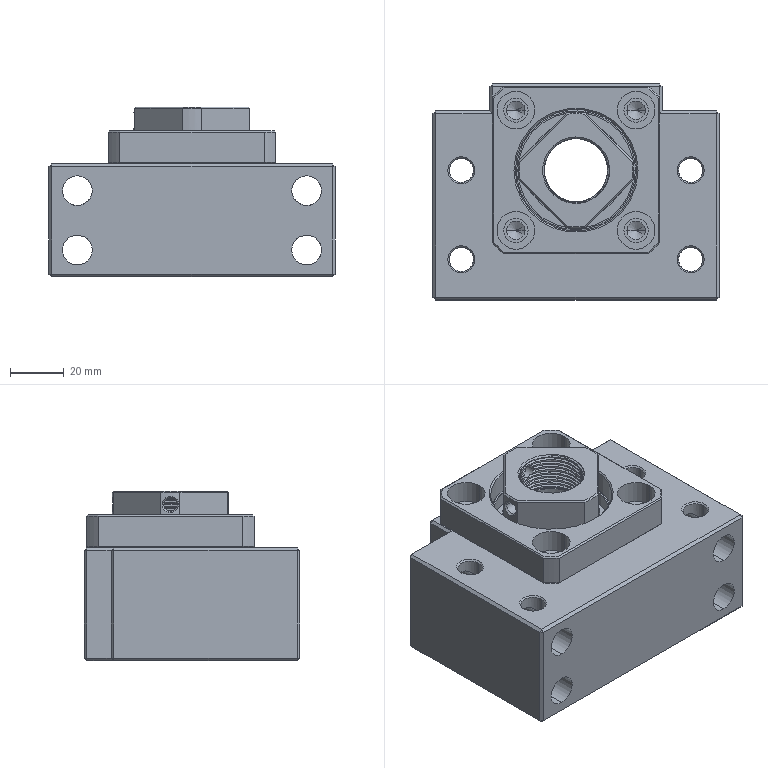Part | SolidWorks | features BaseBody 39 | 39 solids | 491 faces | box 106 x 80 x 63 mm | volume 286934 mm3 | spline 158 | cylinder 156 | plane 103 | cone 74 | commonest cylinder face diameters 9 x32 23.5 x21 43 x9 6.8 x8 11 x8 14 x8